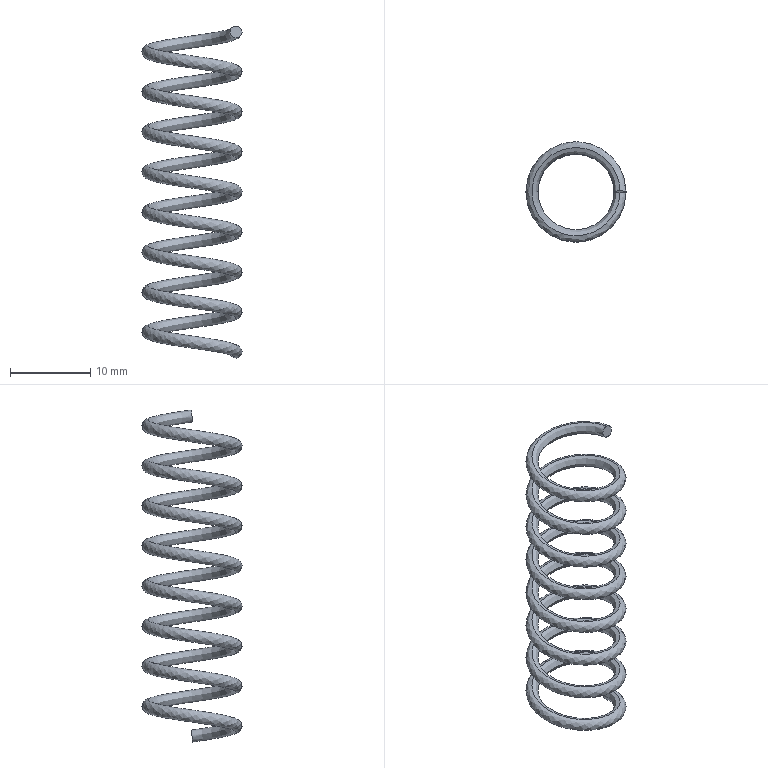Part | SolidWorks | features BaseBody 1 | 1 solid | 4 faces | box 12.5 x 12.5 x 41.485 mm | volume 494.018 mm3 | spline 2 | plane 2